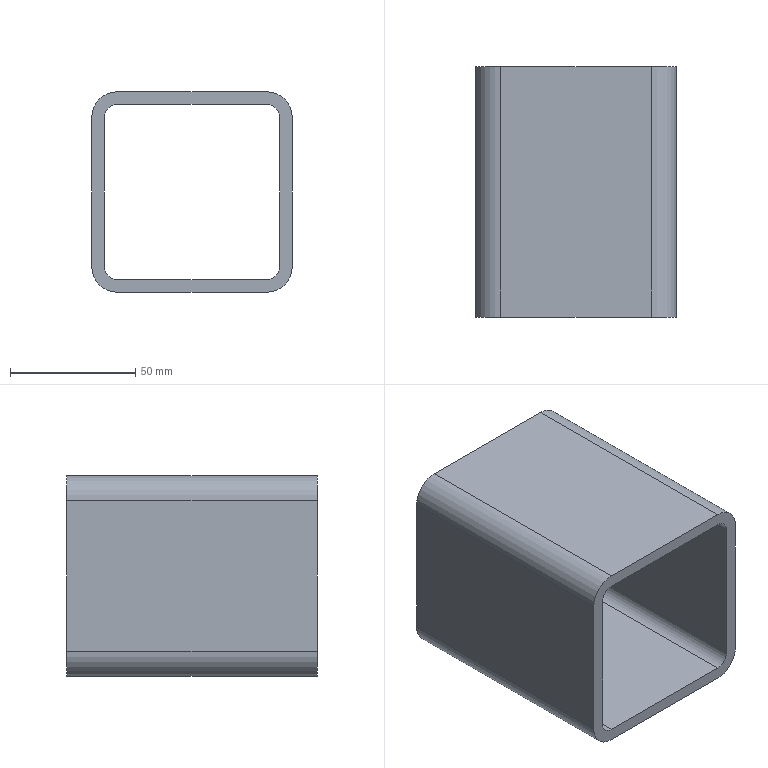Part | SolidWorks | features BaseBody 1 | 1 solid | 18 faces | box 80 x 100 x 80 mm | volume 143562 mm3 | plane 10 | cylinder 8 | commonest cylinder face diameters 10 x4 20 x4
STEP:
#1=CARTESIAN_POINT('',(-40.,0.,30.));
#2=VERTEX_POINT('',#1);
#3=CARTESIAN_POINT('',(-30.,0.,40.));
#4=VERTEX_POINT('',#3);
#5=CARTESIAN_POINT('',(-30.,0.,30.));
#6=DIRECTION('',(0.,1.,0.));
#7=DIRECTION('',(0.,0.,1.));
#8=AXIS2_PLACEMENT_3D('',#5,#6,#7);
#9=CIRCLE('',#8,10.);
#10=EDGE_CURVE('',#2,#4,#9,.T.);
#11=ORIENTED_EDGE('',*,*,#10,.T.);
#12=CARTESIAN_POINT('',(-30.,100.,40.));
#13=VERTEX_POINT('',#12);
#14=CARTESIAN_POINT('',(-30.,100.,40.));
#15=DIRECTION('',(0.,-1.,0.));
#16=VECTOR('',#15,1000.);
#17=LINE('',#14,#16);
#18=EDGE_CURVE('',#13,#4,#17,.T.);
#19=ORIENTED_EDGE('',*,*,#18,.F.);
#20=CARTESIAN_POINT('',(-40.,100.,30.));
#21=VERTEX_POINT('',#20);
#22=CARTESIAN_POINT('',(-30.,100.,30.));
#23=DIRECTION('',(0.,1.,0.));
#24=DIRECTION('',(0.,0.,1.));
#25=AXIS2_PLACEMENT_3D('',#22,#23,#24);
#26=CIRCLE('',#25,10.);
#27=EDGE_CURVE('',#21,#13,#26,.T.);
#28=ORIENTED_EDGE('',*,*,#27,.F.);
#29=CARTESIAN_POINT('',(-40.,100.,30.));
#30=DIRECTION('',(0.,-1.,0.));
#31=VECTOR('',#30,1000.);
#32=LINE('',#29,#31);
#33=EDGE_CURVE('',#21,#2,#32,.T.);
#34=ORIENTED_EDGE('',*,*,#33,.T.);
#35=EDGE_LOOP('',(#11,#19,#28,#34));
#36=FACE_OUTER_BOUND('',#35,.T.);
#37=CARTESIAN_POINT('',(-30.,100.,30.));
#38=DIRECTION('',(0.,-1.,0.));
#39=DIRECTION('',(0.,0.,-1.));
#40=AXIS2_PLACEMENT_3D('',#37,#38,#39);
#41=CYLINDRICAL_SURFACE('',#40,10.);
#42=ADVANCED_FACE('',(#36),#41,.T.);
#43=CARTESIAN_POINT('',(30.,0.,40.));
#44=VERTEX_POINT('',#43);
#45=CARTESIAN_POINT('',(-30.,0.,40.));
#46=DIRECTION('',(1.,0.,0.));
#47=VECTOR('',#46,1000.);
#48=LINE('',#45,#47);
#49=EDGE_CURVE('',#4,#44,#48,.T.);
#50=ORIENTED_EDGE('',*,*,#49,.T.);
#51=CARTESIAN_POINT('',(30.,100.,40.));
#52=VERTEX_POINT('',#51);
#53=CARTESIAN_POINT('',(30.,100.,40.));
#54=DIRECTION('',(0.,-1.,0.));
#55=VECTOR('',#54,1000.);
#56=LINE('',#53,#55);
#57=EDGE_CURVE('',#52,#44,#56,.T.);
#58=ORIENTED_EDGE('',*,*,#57,.F.);
#59=CARTESIAN_POINT('',(-30.,100.,40.));
#60=DIRECTION('',(1.,0.,0.));
#61=VECTOR('',#60,1000.);
#62=LINE('',#59,#61);
#63=EDGE_CURVE('',#13,#52,#62,.T.);
#64=ORIENTED_EDGE('',*,*,#63,.F.);
#65=ORIENTED_EDGE('',*,*,#18,.T.);
#66=EDGE_LOOP('',(#50,#58,#64,#65));
#67=FACE_OUTER_BOUND('',#66,.T.);
#68=CARTESIAN_POINT('',(-30.,100.,40.));
#69=DIRECTION('',(0.,0.,-1.));
#70=DIRECTION('',(-1.,0.,0.));
#71=AXIS2_PLACEMENT_3D('',#68,#69,#70);
#72=PLANE('',#71);
#73=ADVANCED_FACE('',(#67),#72,.F.);
#74=CARTESIAN_POINT('',(40.,0.,30.));
#75=VERTEX_POINT('',#74);
#76=CARTESIAN_POINT('',(30.,0.,30.));
#77=DIRECTION('',(0.,1.,0.));
#78=DIRECTION('',(0.,0.,1.));
#79=AXIS2_PLACEMENT_3D('',#76,#77,#78);
#80=CIRCLE('',#79,10.);
#81=EDGE_CURVE('',#44,#75,#80,.T.);
#82=ORIENTED_EDGE('',*,*,#81,.T.);
#83=CARTESIAN_POINT('',(40.,100.,30.));
#84=VERTEX_POINT('',#83);
#85=CARTESIAN_POINT('',(40.,100.,30.));
#86=DIRECTION('',(0.,-1.,0.));
#87=VECTOR('',#86,1000.);
#88=LINE('',#85,#87);
#89=EDGE_CURVE('',#84,#75,#88,.T.);
#90=ORIENTED_EDGE('',*,*,#89,.F.);
#91=CARTESIAN_POINT('',(30.,100.,30.));
#92=DIRECTION('',(0.,1.,0.));
#93=DIRECTION('',(0.,0.,1.));
#94=AXIS2_PLACEMENT_3D('',#91,#92,#93);
#95=CIRCLE('',#94,10.);
#96=EDGE_CURVE('',#52,#84,#95,.T.);
#97=ORIENTED_EDGE('',*,*,#96,.F.);
#98=ORIENTED_EDGE('',*,*,#57,.T.);
#99=EDGE_LOOP('',(#82,#90,#97,#98));
#100=FACE_OUTER_BOUND('',#99,.T.);
#101=CARTESIAN_POINT('',(30.,100.,30.));
#102=DIRECTION('',(0.,-1.,0.));
#103=DIRECTION('',(0.,0.,-1.));
#104=AXIS2_PLACEMENT_3D('',#101,#102,#103);
#105=CYLINDRICAL_SURFACE('',#104,10.);
#106=ADVANCED_FACE('',(#100),#105,.T.);
#107=CARTESIAN_POINT('',(40.,0.,-30.));
#108=VERTEX_POINT('',#107);
#109=CARTESIAN_POINT('',(40.,0.,-30.));
#110=DIRECTION('',(0.,0.,-1.));
#111=VECTOR('',#110,1000.);
#112=LINE('',#109,#111);
#113=EDGE_CURVE('',#75,#108,#112,.T.);
#114=ORIENTED_EDGE('',*,*,#113,.T.);
#115=CARTESIAN_POINT('',(40.,100.,-30.));
#116=VERTEX_POINT('',#115);
#117=CARTESIAN_POINT('',(40.,100.,-30.));
#118=DIRECTION('',(0.,-1.,0.));
#119=VECTOR('',#118,1000.);
#120=LINE('',#117,#119);
#121=EDGE_CURVE('',#116,#108,#120,.T.);
#122=ORIENTED_EDGE('',*,*,#121,.F.);
#123=CARTESIAN_POINT('',(40.,100.,-30.));
#124=DIRECTION('',(0.,0.,-1.));
#125=VECTOR('',#124,1000.);
#126=LINE('',#123,#125);
#127=EDGE_CURVE('',#84,#116,#126,.T.);
#128=ORIENTED_EDGE('',*,*,#127,.F.);
#129=ORIENTED_EDGE('',*,*,#89,.T.);
#130=EDGE_LOOP('',(#114,#122,#128,#129));
#131=FACE_OUTER_BOUND('',#130,.T.);
#132=CARTESIAN_POINT('',(40.,100.,-30.));
#133=DIRECTION('',(-1.,0.,0.));
#134=DIRECTION('',(0.,0.,1.));
#135=AXIS2_PLACEMENT_3D('',#132,#133,#134);
#136=PLANE('',#135);
#137=ADVANCED_FACE('',(#131),#136,.F.);
#138=CARTESIAN_POINT('',(30.,0.,-40.));
#139=VERTEX_POINT('',#138);
#140=CARTESIAN_POINT('',(30.,0.,-30.));
#141=DIRECTION('',(0.,1.,0.));
#142=DIRECTION('',(0.,0.,1.));
#143=AXIS2_PLACEMENT_3D('',#140,#141,#142);
#144=CIRCLE('',#143,10.);
#145=EDGE_CURVE('',#108,#139,#144,.T.);
#146=ORIENTED_EDGE('',*,*,#145,.T.);
#147=CARTESIAN_POINT('',(30.,100.,-40.));
#148=VERTEX_POINT('',#147);
#149=CARTESIAN_POINT('',(30.,100.,-40.));
#150=DIRECTION('',(0.,-1.,0.));
#151=VECTOR('',#150,1000.);
#152=LINE('',#149,#151);
#153=EDGE_CURVE('',#148,#139,#152,.T.);
#154=ORIENTED_EDGE('',*,*,#153,.F.);
#155=CARTESIAN_POINT('',(30.,100.,-30.));
#156=DIRECTION('',(0.,1.,0.));
#157=DIRECTION('',(0.,0.,1.));
#158=AXIS2_PLACEMENT_3D('',#155,#156,#157);
#159=CIRCLE('',#158,10.);
#160=EDGE_CURVE('',#116,#148,#159,.T.);
#161=ORIENTED_EDGE('',*,*,#160,.F.);
#162=ORIENTED_EDGE('',*,*,#121,.T.);
#163=EDGE_LOOP('',(#146,#154,#161,#162));
#164=FACE_OUTER_BOUND('',#163,.T.);
#165=CARTESIAN_POINT('',(30.,100.,-30.));
#166=DIRECTION('',(0.,-1.,0.));
#167=DIRECTION('',(0.,0.,-1.));
#168=AXIS2_PLACEMENT_3D('',#165,#166,#167);
#169=CYLINDRICAL_SURFACE('',#168,10.);
#170=ADVANCED_FACE('',(#164),#169,.T.);
#171=CARTESIAN_POINT('',(-30.,0.,-40.));
#172=VERTEX_POINT('',#171);
#173=CARTESIAN_POINT('',(30.,0.,-40.));
#174=DIRECTION('',(-1.,0.,0.));
#175=VECTOR('',#174,1000.);
#176=LINE('',#173,#175);
#177=EDGE_CURVE('',#139,#172,#176,.T.);
#178=ORIENTED_EDGE('',*,*,#177,.T.);
#179=CARTESIAN_POINT('',(-30.,100.,-40.));
#180=VERTEX_POINT('',#179);
#181=CARTESIAN_POINT('',(-30.,100.,-40.));
#182=DIRECTION('',(0.,-1.,0.));
#183=VECTOR('',#182,1000.);
#184=LINE('',#181,#183);
#185=EDGE_CURVE('',#180,#172,#184,.T.);
#186=ORIENTED_EDGE('',*,*,#185,.F.);
#187=CARTESIAN_POINT('',(30.,100.,-40.));
#188=DIRECTION('',(-1.,0.,0.));
#189=VECTOR('',#188,1000.);
#190=LINE('',#187,#189);
#191=EDGE_CURVE('',#148,#180,#190,.T.);
#192=ORIENTED_EDGE('',*,*,#191,.F.);
#193=ORIENTED_EDGE('',*,*,#153,.T.);
#194=EDGE_LOOP('',(#178,#186,#192,#193));
#195=FACE_OUTER_BOUND('',#194,.T.);
#196=CARTESIAN_POINT('',(30.,100.,-40.));
#197=DIRECTION('',(0.,0.,1.));
#198=DIRECTION('',(1.,0.,0.));
#199=AXIS2_PLACEMENT_3D('',#196,#197,#198);
#200=PLANE('',#199);
#201=ADVANCED_FACE('',(#195),#200,.F.);
#202=CARTESIAN_POINT('',(-40.,0.,-30.));
#203=VERTEX_POINT('',#202);
#204=CARTESIAN_POINT('',(-30.,0.,-30.));
#205=DIRECTION('',(0.,1.,0.));
#206=DIRECTION('',(0.,0.,1.));
#207=AXIS2_PLACEMENT_3D('',#204,#205,#206);
#208=CIRCLE('',#207,10.);
#209=EDGE_CURVE('',#172,#203,#208,.T.);
#210=ORIENTED_EDGE('',*,*,#209,.T.);
#211=CARTESIAN_POINT('',(-40.,100.,-30.));
#212=VERTEX_POINT('',#211);
#213=CARTESIAN_POINT('',(-40.,100.,-30.));
#214=DIRECTION('',(0.,-1.,0.));
#215=VECTOR('',#214,1000.);
#216=LINE('',#213,#215);
#217=EDGE_CURVE('',#212,#203,#216,.T.);
#218=ORIENTED_EDGE('',*,*,#217,.F.);
#219=CARTESIAN_POINT('',(-30.,100.,-30.));
#220=DIRECTION('',(0.,1.,0.));
#221=DIRECTION('',(0.,0.,1.));
#222=AXIS2_PLACEMENT_3D('',#219,#220,#221);
#223=CIRCLE('',#222,10.);
#224=EDGE_CURVE('',#180,#212,#223,.T.);
#225=ORIENTED_EDGE('',*,*,#224,.F.);
#226=ORIENTED_EDGE('',*,*,#185,.T.);
#227=EDGE_LOOP('',(#210,#218,#225,#226));
#228=FACE_OUTER_BOUND('',#227,.T.);
#229=CARTESIAN_POINT('',(-30.,100.,-30.));
#230=DIRECTION('',(0.,-1.,0.));
#231=DIRECTION('',(0.,0.,-1.));
#232=AXIS2_PLACEMENT_3D('',#229,#230,#231);
#233=CYLINDRICAL_SURFACE('',#232,10.);
#234=ADVANCED_FACE('',(#228),#233,.T.);
#235=CARTESIAN_POINT('',(30.,0.,35.));
#236=VERTEX_POINT('',#235);
#237=CARTESIAN_POINT('',(35.,0.,30.));
#238=VERTEX_POINT('',#237);
#239=CARTESIAN_POINT('',(30.,0.,30.));
#240=DIRECTION('',(0.,1.,0.));
#241=DIRECTION('',(0.,0.,1.));
#242=AXIS2_PLACEMENT_3D('',#239,#240,#241);
#243=CIRCLE('',#242,5.);
#244=EDGE_CURVE('',#236,#238,#243,.T.);
#245=ORIENTED_EDGE('',*,*,#244,.F.);
#246=CARTESIAN_POINT('',(30.,100.,35.));
#247=VERTEX_POINT('',#246);
#248=CARTESIAN_POINT('',(30.,100.,35.));
#249=DIRECTION('',(0.,-1.,0.));
#250=VECTOR('',#249,1000.);
#251=LINE('',#248,#250);
#252=EDGE_CURVE('',#247,#236,#251,.T.);
#253=ORIENTED_EDGE('',*,*,#252,.F.);
#254=CARTESIAN_POINT('',(35.,100.,30.));
#255=VERTEX_POINT('',#254);
#256=CARTESIAN_POINT('',(30.,100.,30.));
#257=DIRECTION('',(0.,1.,0.));
#258=DIRECTION('',(0.,0.,1.));
#259=AXIS2_PLACEMENT_3D('',#256,#257,#258);
#260=CIRCLE('',#259,5.);
#261=EDGE_CURVE('',#247,#255,#260,.T.);
#262=ORIENTED_EDGE('',*,*,#261,.T.);
#263=CARTESIAN_POINT('',(35.,100.,30.));
#264=DIRECTION('',(0.,-1.,0.));
#265=VECTOR('',#264,1000.);
#266=LINE('',#263,#265);
#267=EDGE_CURVE('',#255,#238,#266,.T.);
#268=ORIENTED_EDGE('',*,*,#267,.T.);
#269=EDGE_LOOP('',(#245,#253,#262,#268));
#270=FACE_OUTER_BOUND('',#269,.T.);
#271=CARTESIAN_POINT('',(30.,100.,30.));
#272=DIRECTION('',(0.,-1.,0.));
#273=DIRECTION('',(0.,0.,-1.));
#274=AXIS2_PLACEMENT_3D('',#271,#272,#273);
#275=CYLINDRICAL_SURFACE('',#274,5.);
#276=ADVANCED_FACE('',(#270),#275,.F.);
#277=CARTESIAN_POINT('',(-30.,0.,35.));
#278=VERTEX_POINT('',#277);
#279=CARTESIAN_POINT('',(-30.,0.,35.));
#280=DIRECTION('',(1.,0.,0.));
#281=VECTOR('',#280,1000.);
#282=LINE('',#279,#281);
#283=EDGE_CURVE('',#278,#236,#282,.T.);
#284=ORIENTED_EDGE('',*,*,#283,.F.);
#285=CARTESIAN_POINT('',(-30.,100.,35.));
#286=VERTEX_POINT('',#285);
#287=CARTESIAN_POINT('',(-30.,100.,35.));
#288=DIRECTION('',(0.,-1.,0.));
#289=VECTOR('',#288,1000.);
#290=LINE('',#287,#289);
#291=EDGE_CURVE('',#286,#278,#290,.T.);
#292=ORIENTED_EDGE('',*,*,#291,.F.);
#293=CARTESIAN_POINT('',(-30.,100.,35.));
#294=DIRECTION('',(1.,0.,0.));
#295=VECTOR('',#294,1000.);
#296=LINE('',#293,#295);
#297=EDGE_CURVE('',#286,#247,#296,.T.);
#298=ORIENTED_EDGE('',*,*,#297,.T.);
#299=ORIENTED_EDGE('',*,*,#252,.T.);
#300=EDGE_LOOP('',(#284,#292,#298,#299));
#301=FACE_OUTER_BOUND('',#300,.T.);
#302=CARTESIAN_POINT('',(-30.,100.,35.));
#303=DIRECTION('',(0.,0.,-1.));
#304=DIRECTION('',(-1.,0.,0.));
#305=AXIS2_PLACEMENT_3D('',#302,#303,#304);
#306=PLANE('',#305);
#307=ADVANCED_FACE('',(#301),#306,.T.);
#308=CARTESIAN_POINT('',(-35.,0.,30.));
#309=VERTEX_POINT('',#308);
#310=CARTESIAN_POINT('',(-30.,0.,30.));
#311=DIRECTION('',(0.,1.,0.));
#312=DIRECTION('',(0.,0.,1.));
#313=AXIS2_PLACEMENT_3D('',#310,#311,#312);
#314=CIRCLE('',#313,5.);
#315=EDGE_CURVE('',#309,#278,#314,.T.);
#316=ORIENTED_EDGE('',*,*,#315,.F.);
#317=CARTESIAN_POINT('',(-35.,100.,30.));
#318=VERTEX_POINT('',#317);
#319=CARTESIAN_POINT('',(-35.,100.,30.));
#320=DIRECTION('',(0.,-1.,0.));
#321=VECTOR('',#320,1000.);
#322=LINE('',#319,#321);
#323=EDGE_CURVE('',#318,#309,#322,.T.);
#324=ORIENTED_EDGE('',*,*,#323,.F.);
#325=CARTESIAN_POINT('',(-30.,100.,30.));
#326=DIRECTION('',(0.,1.,0.));
#327=DIRECTION('',(0.,0.,1.));
#328=AXIS2_PLACEMENT_3D('',#325,#326,#327);
#329=CIRCLE('',#328,5.);
#330=EDGE_CURVE('',#318,#286,#329,.T.);
#331=ORIENTED_EDGE('',*,*,#330,.T.);
#332=ORIENTED_EDGE('',*,*,#291,.T.);
#333=EDGE_LOOP('',(#316,#324,#331,#332));
#334=FACE_OUTER_BOUND('',#333,.T.);
#335=CARTESIAN_POINT('',(-30.,100.,30.));
#336=DIRECTION('',(0.,-1.,0.));
#337=DIRECTION('',(0.,0.,-1.));
#338=AXIS2_PLACEMENT_3D('',#335,#336,#337);
#339=CYLINDRICAL_SURFACE('',#338,5.);
#340=ADVANCED_FACE('',(#334),#339,.F.);
#341=CARTESIAN_POINT('',(-35.,0.,-30.));
#342=VERTEX_POINT('',#341);
#343=CARTESIAN_POINT('',(-35.,0.,30.));
#344=DIRECTION('',(0.,0.,1.));
#345=VECTOR('',#344,1000.);
#346=LINE('',#343,#345);
#347=EDGE_CURVE('',#342,#309,#346,.T.);
#348=ORIENTED_EDGE('',*,*,#347,.F.);
#349=CARTESIAN_POINT('',(-35.,100.,-30.));
#350=VERTEX_POINT('',#349);
#351=CARTESIAN_POINT('',(-35.,100.,-30.));
#352=DIRECTION('',(0.,-1.,0.));
#353=VECTOR('',#352,1000.);
#354=LINE('',#351,#353);
#355=EDGE_CURVE('',#350,#342,#354,.T.);
#356=ORIENTED_EDGE('',*,*,#355,.F.);
#357=CARTESIAN_POINT('',(-35.,100.,30.));
#358=DIRECTION('',(0.,0.,1.));
#359=VECTOR('',#358,1000.);
#360=LINE('',#357,#359);
#361=EDGE_CURVE('',#350,#318,#360,.T.);
#362=ORIENTED_EDGE('',*,*,#361,.T.);
#363=ORIENTED_EDGE('',*,*,#323,.T.);
#364=EDGE_LOOP('',(#348,#356,#362,#363));
#365=FACE_OUTER_BOUND('',#364,.T.);
#366=CARTESIAN_POINT('',(-35.,100.,30.));
#367=DIRECTION('',(1.,0.,0.));
#368=DIRECTION('',(0.,0.,-1.));
#369=AXIS2_PLACEMENT_3D('',#366,#367,#368);
#370=PLANE('',#369);
#371=ADVANCED_FACE('',(#365),#370,.T.);
#372=CARTESIAN_POINT('',(-30.,0.,-35.));
#373=VERTEX_POINT('',#372);
#374=CARTESIAN_POINT('',(-30.,0.,-30.));
#375=DIRECTION('',(0.,1.,0.));
#376=DIRECTION('',(0.,0.,1.));
#377=AXIS2_PLACEMENT_3D('',#374,#375,#376);
#378=CIRCLE('',#377,5.);
#379=EDGE_CURVE('',#373,#342,#378,.T.);
#380=ORIENTED_EDGE('',*,*,#379,.F.);
#381=CARTESIAN_POINT('',(-30.,100.,-35.));
#382=VERTEX_POINT('',#381);
#383=CARTESIAN_POINT('',(-30.,100.,-35.));
#384=DIRECTION('',(0.,-1.,0.));
#385=VECTOR('',#384,1000.);
#386=LINE('',#383,#385);
#387=EDGE_CURVE('',#382,#373,#386,.T.);
#388=ORIENTED_EDGE('',*,*,#387,.F.);
#389=CARTESIAN_POINT('',(-30.,100.,-30.));
#390=DIRECTION('',(0.,1.,0.));
#391=DIRECTION('',(0.,0.,1.));
#392=AXIS2_PLACEMENT_3D('',#389,#390,#391);
#393=CIRCLE('',#392,5.);
#394=EDGE_CURVE('',#382,#350,#393,.T.);
#395=ORIENTED_EDGE('',*,*,#394,.T.);
#396=ORIENTED_EDGE('',*,*,#355,.T.);
#397=EDGE_LOOP('',(#380,#388,#395,#396));
#398=FACE_OUTER_BOUND('',#397,.T.);
#399=CARTESIAN_POINT('',(-30.,100.,-30.));
#400=DIRECTION('',(0.,-1.,0.));
#401=DIRECTION('',(0.,0.,-1.));
#402=AXIS2_PLACEMENT_3D('',#399,#400,#401);
#403=CYLINDRICAL_SURFACE('',#402,5.);
#404=ADVANCED_FACE('',(#398),#403,.F.);
#405=CARTESIAN_POINT('',(30.,0.,-35.));
#406=VERTEX_POINT('',#405);
#407=CARTESIAN_POINT('',(30.,0.,-35.));
#408=DIRECTION('',(-1.,0.,0.));
#409=VECTOR('',#408,1000.);
#410=LINE('',#407,#409);
#411=EDGE_CURVE('',#406,#373,#410,.T.);
#412=ORIENTED_EDGE('',*,*,#411,.F.);
#413=CARTESIAN_POINT('',(30.,100.,-35.));
#414=VERTEX_POINT('',#413);
#415=CARTESIAN_POINT('',(30.,100.,-35.));
#416=DIRECTION('',(0.,-1.,0.));
#417=VECTOR('',#416,1000.);
#418=LINE('',#415,#417);
#419=EDGE_CURVE('',#414,#406,#418,.T.);
#420=ORIENTED_EDGE('',*,*,#419,.F.);
#421=CARTESIAN_POINT('',(30.,100.,-35.));
#422=DIRECTION('',(-1.,0.,0.));
#423=VECTOR('',#422,1000.);
#424=LINE('',#421,#423);
#425=EDGE_CURVE('',#414,#382,#424,.T.);
#426=ORIENTED_EDGE('',*,*,#425,.T.);
#427=ORIENTED_EDGE('',*,*,#387,.T.);
#428=EDGE_LOOP('',(#412,#420,#426,#427));
#429=FACE_OUTER_BOUND('',#428,.T.);
#430=CARTESIAN_POINT('',(30.,100.,-35.));
#431=DIRECTION('',(0.,0.,1.));
#432=DIRECTION('',(1.,0.,0.));
#433=AXIS2_PLACEMENT_3D('',#430,#431,#432);
#434=PLANE('',#433);
#435=ADVANCED_FACE('',(#429),#434,.T.);
#436=CARTESIAN_POINT('',(35.,0.,-30.));
#437=VERTEX_POINT('',#436);
#438=CARTESIAN_POINT('',(30.,0.,-30.));
#439=DIRECTION('',(0.,1.,0.));
#440=DIRECTION('',(0.,0.,1.));
#441=AXIS2_PLACEMENT_3D('',#438,#439,#440);
#442=CIRCLE('',#441,5.);
#443=EDGE_CURVE('',#437,#406,#442,.T.);
#444=ORIENTED_EDGE('',*,*,#443,.F.);
#445=CARTESIAN_POINT('',(35.,100.,-30.));
#446=VERTEX_POINT('',#445);
#447=CARTESIAN_POINT('',(35.,100.,-30.));
#448=DIRECTION('',(0.,-1.,0.));
#449=VECTOR('',#448,1000.);
#450=LINE('',#447,#449);
#451=EDGE_CURVE('',#446,#437,#450,.T.);
#452=ORIENTED_EDGE('',*,*,#451,.F.);
#453=CARTESIAN_POINT('',(30.,100.,-30.));
#454=DIRECTION('',(0.,1.,0.));
#455=DIRECTION('',(0.,0.,1.));
#456=AXIS2_PLACEMENT_3D('',#453,#454,#455);
#457=CIRCLE('',#456,5.);
#458=EDGE_CURVE('',#446,#414,#457,.T.);
#459=ORIENTED_EDGE('',*,*,#458,.T.);
#460=ORIENTED_EDGE('',*,*,#419,.T.);
#461=EDGE_LOOP('',(#444,#452,#459,#460));
#462=FACE_OUTER_BOUND('',#461,.T.);
#463=CARTESIAN_POINT('',(30.,100.,-30.));
#464=DIRECTION('',(0.,-1.,0.));
#465=DIRECTION('',(0.,0.,-1.));
#466=AXIS2_PLACEMENT_3D('',#463,#464,#465);
#467=CYLINDRICAL_SURFACE('',#466,5.);
#468=ADVANCED_FACE('',(#462),#467,.F.);
#469=CARTESIAN_POINT('',(35.,0.,-30.));
#470=DIRECTION('',(0.,0.,-1.));
#471=VECTOR('',#470,1000.);
#472=LINE('',#469,#471);
#473=EDGE_CURVE('',#238,#437,#472,.T.);
#474=ORIENTED_EDGE('',*,*,#473,.F.);
#475=ORIENTED_EDGE('',*,*,#267,.F.);
#476=CARTESIAN_POINT('',(35.,100.,-30.));
#477=DIRECTION('',(0.,0.,-1.));
#478=VECTOR('',#477,1000.);
#479=LINE('',#476,#478);
#480=EDGE_CURVE('',#255,#446,#479,.T.);
#481=ORIENTED_EDGE('',*,*,#480,.T.);
#482=ORIENTED_EDGE('',*,*,#451,.T.);
#483=EDGE_LOOP('',(#474,#475,#481,#482));
#484=FACE_OUTER_BOUND('',#483,.T.);
#485=CARTESIAN_POINT('',(35.,100.,-30.));
#486=DIRECTION('',(-1.,0.,0.));
#487=DIRECTION('',(0.,0.,1.));
#488=AXIS2_PLACEMENT_3D('',#485,#486,#487);
#489=PLANE('',#488);
#490=ADVANCED_FACE('',(#484),#489,.T.);
#491=CARTESIAN_POINT('',(-40.,0.,30.));
#492=DIRECTION('',(0.,0.,1.));
#493=VECTOR('',#492,1000.);
#494=LINE('',#491,#493);
#495=EDGE_CURVE('',#203,#2,#494,.T.);
#496=ORIENTED_EDGE('',*,*,#495,.T.);
#497=ORIENTED_EDGE('',*,*,#33,.F.);
#498=CARTESIAN_POINT('',(-40.,100.,30.));
#499=DIRECTION('',(0.,0.,1.));
#500=VECTOR('',#499,1000.);
#501=LINE('',#498,#500);
#502=EDGE_CURVE('',#212,#21,#501,.T.);
#503=ORIENTED_EDGE('',*,*,#502,.F.);
#504=ORIENTED_EDGE('',*,*,#217,.T.);
#505=EDGE_LOOP('',(#496,#497,#503,#504));
#506=FACE_OUTER_BOUND('',#505,.T.);
#507=CARTESIAN_POINT('',(-40.,100.,30.));
#508=DIRECTION('',(1.,0.,0.));
#509=DIRECTION('',(0.,0.,-1.));
#510=AXIS2_PLACEMENT_3D('',#507,#508,#509);
#511=PLANE('',#510);
#512=ADVANCED_FACE('',(#506),#511,.F.);
#513=ORIENTED_EDGE('',*,*,#261,.F.);
#514=ORIENTED_EDGE('',*,*,#297,.F.);
#515=ORIENTED_EDGE('',*,*,#330,.F.);
#516=ORIENTED_EDGE('',*,*,#361,.F.);
#517=ORIENTED_EDGE('',*,*,#394,.F.);
#518=ORIENTED_EDGE('',*,*,#425,.F.);
#519=ORIENTED_EDGE('',*,*,#458,.F.);
#520=ORIENTED_EDGE('',*,*,#480,.F.);
#521=EDGE_LOOP('',(#513,#514,#515,#516,#517,#518,#519,#520));
#522=FACE_BOUND('',#521,.T.);
#523=ORIENTED_EDGE('',*,*,#27,.T.);
#524=ORIENTED_EDGE('',*,*,#63,.T.);
#525=ORIENTED_EDGE('',*,*,#96,.T.);
#526=ORIENTED_EDGE('',*,*,#127,.T.);
#527=ORIENTED_EDGE('',*,*,#160,.T.);
#528=ORIENTED_EDGE('',*,*,#191,.T.);
#529=ORIENTED_EDGE('',*,*,#224,.T.);
#530=ORIENTED_EDGE('',*,*,#502,.T.);
#531=EDGE_LOOP('',(#523,#524,#525,#526,#527,#528,#529,#530));
#532=FACE_OUTER_BOUND('',#531,.T.);
#533=CARTESIAN_POINT('',(-30.,100.,30.));
#534=DIRECTION('',(0.,1.,0.));
#535=DIRECTION('',(0.,0.,1.));
#536=AXIS2_PLACEMENT_3D('',#533,#534,#535);
#537=PLANE('',#536);
#538=ADVANCED_FACE('',(#522,#532),#537,.T.);
#539=ORIENTED_EDGE('',*,*,#244,.T.);
#540=ORIENTED_EDGE('',*,*,#473,.T.);
#541=ORIENTED_EDGE('',*,*,#443,.T.);
#542=ORIENTED_EDGE('',*,*,#411,.T.);
#543=ORIENTED_EDGE('',*,*,#379,.T.);
#544=ORIENTED_EDGE('',*,*,#347,.T.);
#545=ORIENTED_EDGE('',*,*,#315,.T.);
#546=ORIENTED_EDGE('',*,*,#283,.T.);
#547=EDGE_LOOP('',(#539,#540,#541,#542,#543,#544,#545,#546));
#548=FACE_BOUND('',#547,.T.);
#549=ORIENTED_EDGE('',*,*,#10,.F.);
#550=ORIENTED_EDGE('',*,*,#495,.F.);
#551=ORIENTED_EDGE('',*,*,#209,.F.);
#552=ORIENTED_EDGE('',*,*,#177,.F.);
#553=ORIENTED_EDGE('',*,*,#145,.F.);
#554=ORIENTED_EDGE('',*,*,#113,.F.);
#555=ORIENTED_EDGE('',*,*,#81,.F.);
#556=ORIENTED_EDGE('',*,*,#49,.F.);
#557=EDGE_LOOP('',(#549,#550,#551,#552,#553,#554,#555,#556));
#558=FACE_OUTER_BOUND('',#557,.T.);
#559=CARTESIAN_POINT('',(-30.,0.,30.));
#560=DIRECTION('',(0.,1.,0.));
#561=DIRECTION('',(0.,0.,1.));
#562=AXIS2_PLACEMENT_3D('',#559,#560,#561);
#563=PLANE('',#562);
#564=ADVANCED_FACE('',(#548,#558),#563,.F.);
#565=CLOSED_SHELL('',(#42,#73,#106,#137,#170,#201,#234,#276,#307,#340,#371,#404,#435,#468,#490,#512,#538,#564));
#566=MANIFOLD_SOLID_BREP('',#565);
#567=CARTESIAN_POINT('',(0.,0.,0.));
#568=DIRECTION('',(0.,0.,1.));
#569=DIRECTION('',(1.,0.,0.));
#570=AXIS2_PLACEMENT_3D('',#567,#568,#569);
#571=(LENGTH_UNIT()NAMED_UNIT(*)SI_UNIT(.MILLI.,.METRE.));
#572=UNCERTAINTY_MEASURE_WITH_UNIT(LENGTH_MEASURE(0.00001),#571,'','');
#573=(NAMED_UNIT(*)PLANE_ANGLE_UNIT()SI_UNIT($,.RADIAN.));
#574=(NAMED_UNIT(*)SI_UNIT($,.STERADIAN.)SOLID_ANGLE_UNIT());
#575=(GEOMETRIC_REPRESENTATION_CONTEXT(3)GLOBAL_UNCERTAINTY_ASSIGNED_CONTEXT((#572))GLOBAL_UNIT_ASSIGNED_CONTEXT((#571,#573,#574))REPRESENTATION_CONTEXT('',''));
#576=ADVANCED_BREP_SHAPE_REPRESENTATION('',(#566,#570),#575);